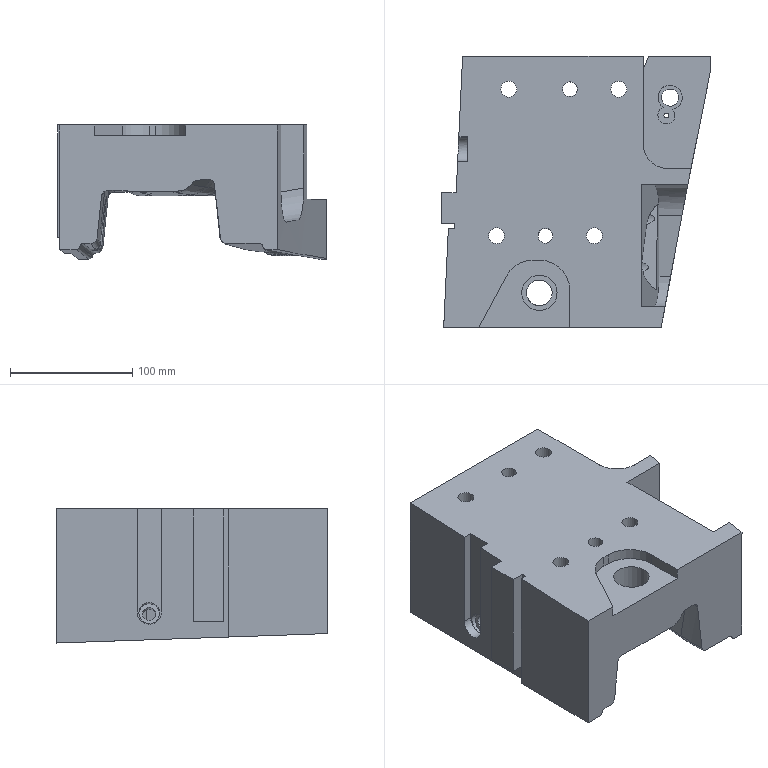Part | NX | features solid 2 | 1 solid | 170 faces | box 220 x 221.783 x 109.751 mm | volume 2466249 mm3 | spline 103 | plane 35 | cylinder 32 | commonest cylinder face diameters 20 x8 50 x8 13 x4 12 x2 14 x2 16 x2